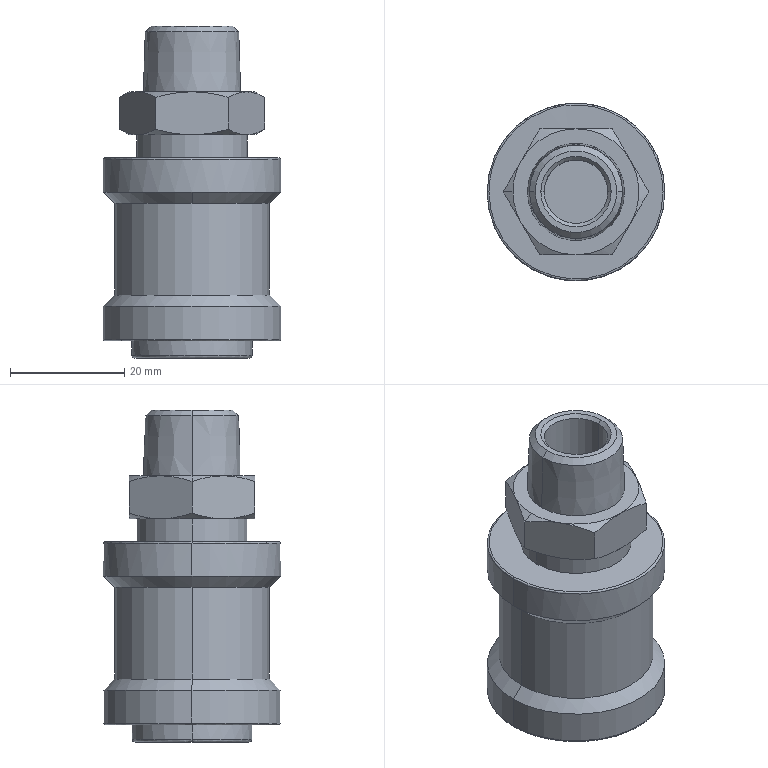Part | STEP file | VL3ME | 1 solid | 60 faces | box 31 x 31 x 58 mm | volume 23537 mm3 | cone 28 | plane 14 | cylinder 12 | spline 6 | commonest cylinder face diameters 31 x4 11.108 x2 19.331 x2 21 x2 27 x2